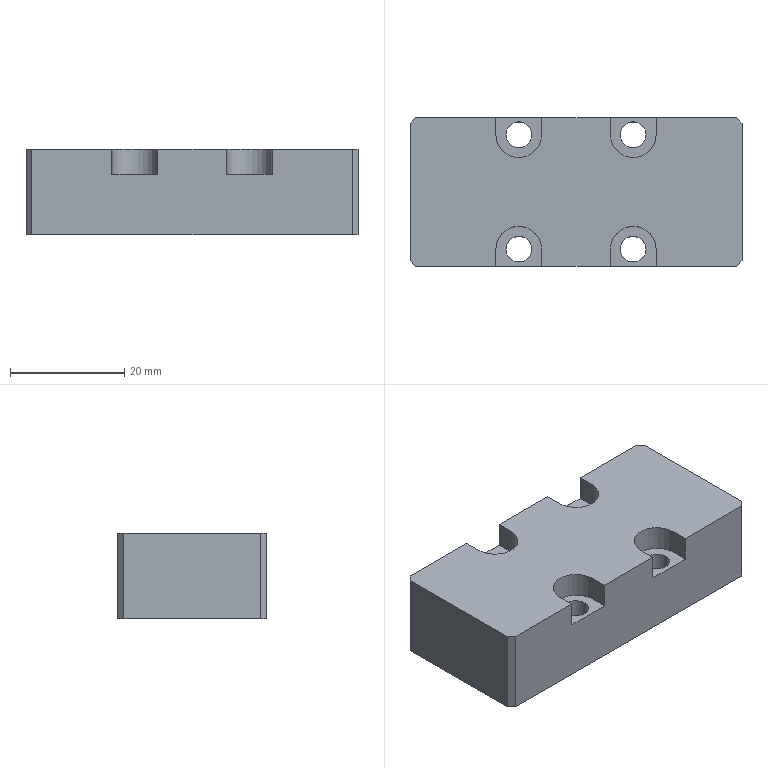Part | SolidWorks | features HoleWzd 2, Chamfer 1, Extrusion 1, ICE 1, MirrorPattern 1 | 1 solid | 42 faces | box 58 x 26 x 15 mm | volume 20953 mm3 | plane 22 | cylinder 16 | cone 4 | commonest cylinder face diameters 4.5 x8 5 x4 8 x4
STEP:
#1=CARTESIAN_POINT('',(15.,0.,-5.5));
#2=VERTEX_POINT('',#1);
#3=CARTESIAN_POINT('',(10.,0.,-5.5));
#4=VERTEX_POINT('',#3);
#5=CARTESIAN_POINT('',(12.5,0.,-5.5));
#6=DIRECTION('',(0.,0.,-1.));
#7=DIRECTION('',(-1.,0.,0.));
#8=AXIS2_PLACEMENT_3D('',#5,#6,#7);
#9=CIRCLE('',#8,2.5);
#10=EDGE_CURVE('',#2,#4,#9,.T.);
#11=ORIENTED_EDGE('',*,*,#10,.F.);
#12=CARTESIAN_POINT('',(15.,0.,-7.5));
#13=VERTEX_POINT('',#12);
#14=CARTESIAN_POINT('',(15.,0.,-7.5));
#15=DIRECTION('',(0.,0.,-1.));
#16=VECTOR('',#15,1000.);
#17=LINE('',#14,#16);
#18=EDGE_CURVE('',#2,#13,#17,.T.);
#19=ORIENTED_EDGE('',*,*,#18,.T.);
#20=CARTESIAN_POINT('',(10.,0.,-7.5));
#21=VERTEX_POINT('',#20);
#22=CARTESIAN_POINT('',(12.5,0.,-7.5));
#23=DIRECTION('',(0.,0.,-1.));
#24=DIRECTION('',(-1.,0.,0.));
#25=AXIS2_PLACEMENT_3D('',#22,#23,#24);
#26=CIRCLE('',#25,2.5);
#27=EDGE_CURVE('',#13,#21,#26,.T.);
#28=ORIENTED_EDGE('',*,*,#27,.T.);
#29=CARTESIAN_POINT('',(10.,0.,-7.5));
#30=DIRECTION('',(0.,0.,-1.));
#31=VECTOR('',#30,1000.);
#32=LINE('',#29,#31);
#33=EDGE_CURVE('',#4,#21,#32,.T.);
#34=ORIENTED_EDGE('',*,*,#33,.F.);
#35=EDGE_LOOP('',(#11,#19,#28,#34));
#36=FACE_OUTER_BOUND('',#35,.T.);
#37=CARTESIAN_POINT('',(12.5,0.,-7.5));
#38=DIRECTION('',(0.,0.,-1.));
#39=DIRECTION('',(-1.,0.,0.));
#40=AXIS2_PLACEMENT_3D('',#37,#38,#39);
#41=CYLINDRICAL_SURFACE('',#40,2.5);
#42=ADVANCED_FACE('',(#36),#41,.F.);
#43=CARTESIAN_POINT('',(12.5,0.,-3.998));
#44=VERTEX_POINT('',#43);
#45=CARTESIAN_POINT('',(10.,0.,-5.5));
#46=DIRECTION('',(-0.8572,0.,-0.515));
#47=VECTOR('',#46,1000.);
#48=LINE('',#45,#47);
#49=EDGE_CURVE('',#44,#4,#48,.T.);
#50=ORIENTED_EDGE('',*,*,#49,.F.);
#51=CARTESIAN_POINT('',(15.,0.,-5.5));
#52=DIRECTION('',(0.8572,0.,-0.515));
#53=VECTOR('',#52,1000.);
#54=LINE('',#51,#53);
#55=EDGE_CURVE('',#44,#2,#54,.T.);
#56=ORIENTED_EDGE('',*,*,#55,.T.);
#57=ORIENTED_EDGE('',*,*,#10,.T.);
#58=EDGE_LOOP('',(#50,#56,#57));
#59=FACE_OUTER_BOUND('',#58,.T.);
#60=CARTESIAN_POINT('',(12.5,0.,-5.5));
#61=DIRECTION('',(0.,0.,-1.));
#62=DIRECTION('',(-1.,0.,0.));
#63=AXIS2_PLACEMENT_3D('',#60,#61,#62);
#64=CONICAL_SURFACE('',#63,2.5,1.03);
#65=ADVANCED_FACE('',(#59),#64,.F.);
#66=CARTESIAN_POINT('',(-10.,0.,-5.5));
#67=VERTEX_POINT('',#66);
#68=CARTESIAN_POINT('',(-15.,0.,-5.5));
#69=VERTEX_POINT('',#68);
#70=CARTESIAN_POINT('',(-12.5,0.,-5.5));
#71=DIRECTION('',(0.,0.,-1.));
#72=DIRECTION('',(-1.,0.,0.));
#73=AXIS2_PLACEMENT_3D('',#70,#71,#72);
#74=CIRCLE('',#73,2.5);
#75=EDGE_CURVE('',#67,#69,#74,.T.);
#76=ORIENTED_EDGE('',*,*,#75,.F.);
#77=CARTESIAN_POINT('',(-10.,0.,-7.5));
#78=VERTEX_POINT('',#77);
#79=CARTESIAN_POINT('',(-10.,0.,-7.5));
#80=DIRECTION('',(0.,0.,-1.));
#81=VECTOR('',#80,1000.);
#82=LINE('',#79,#81);
#83=EDGE_CURVE('',#67,#78,#82,.T.);
#84=ORIENTED_EDGE('',*,*,#83,.T.);
#85=CARTESIAN_POINT('',(-15.,0.,-7.5));
#86=VERTEX_POINT('',#85);
#87=CARTESIAN_POINT('',(-12.5,0.,-7.5));
#88=DIRECTION('',(0.,0.,-1.));
#89=DIRECTION('',(-1.,0.,0.));
#90=AXIS2_PLACEMENT_3D('',#87,#88,#89);
#91=CIRCLE('',#90,2.5);
#92=EDGE_CURVE('',#78,#86,#91,.T.);
#93=ORIENTED_EDGE('',*,*,#92,.T.);
#94=CARTESIAN_POINT('',(-15.,0.,-7.5));
#95=DIRECTION('',(0.,0.,-1.));
#96=VECTOR('',#95,1000.);
#97=LINE('',#94,#96);
#98=EDGE_CURVE('',#69,#86,#97,.T.);
#99=ORIENTED_EDGE('',*,*,#98,.F.);
#100=EDGE_LOOP('',(#76,#84,#93,#99));
#101=FACE_OUTER_BOUND('',#100,.T.);
#102=CARTESIAN_POINT('',(-12.5,0.,-7.5));
#103=DIRECTION('',(0.,0.,-1.));
#104=DIRECTION('',(-1.,0.,0.));
#105=AXIS2_PLACEMENT_3D('',#102,#103,#104);
#106=CYLINDRICAL_SURFACE('',#105,2.5);
#107=ADVANCED_FACE('',(#101),#106,.F.);
#108=CARTESIAN_POINT('',(-12.5,0.,-3.998));
#109=VERTEX_POINT('',#108);
#110=CARTESIAN_POINT('',(-15.,0.,-5.5));
#111=DIRECTION('',(-0.8572,0.,-0.515));
#112=VECTOR('',#111,1000.);
#113=LINE('',#110,#112);
#114=EDGE_CURVE('',#109,#69,#113,.T.);
#115=ORIENTED_EDGE('',*,*,#114,.F.);
#116=CARTESIAN_POINT('',(-10.,0.,-5.5));
#117=DIRECTION('',(0.8572,0.,-0.515));
#118=VECTOR('',#117,1000.);
#119=LINE('',#116,#118);
#120=EDGE_CURVE('',#109,#67,#119,.T.);
#121=ORIENTED_EDGE('',*,*,#120,.T.);
#122=ORIENTED_EDGE('',*,*,#75,.T.);
#123=EDGE_LOOP('',(#115,#121,#122));
#124=FACE_OUTER_BOUND('',#123,.T.);
#125=CARTESIAN_POINT('',(-12.5,0.,-5.5));
#126=DIRECTION('',(0.,0.,-1.));
#127=DIRECTION('',(-1.,0.,0.));
#128=AXIS2_PLACEMENT_3D('',#125,#126,#127);
#129=CONICAL_SURFACE('',#128,2.5,1.03);
#130=ADVANCED_FACE('',(#124),#129,.F.);
#131=CARTESIAN_POINT('',(-12.25,10.,-7.5));
#132=VERTEX_POINT('',#131);
#133=CARTESIAN_POINT('',(-7.75,10.,-7.5));
#134=VERTEX_POINT('',#133);
#135=CARTESIAN_POINT('',(-10.,10.,-7.5));
#136=DIRECTION('',(0.,0.,1.));
#137=DIRECTION('',(1.,0.,0.));
#138=AXIS2_PLACEMENT_3D('',#135,#136,#137);
#139=CIRCLE('',#138,2.25);
#140=EDGE_CURVE('',#132,#134,#139,.T.);
#141=ORIENTED_EDGE('',*,*,#140,.F.);
#142=CARTESIAN_POINT('',(-12.25,10.,3.1));
#143=VERTEX_POINT('',#142);
#144=CARTESIAN_POINT('',(-12.25,10.,7.5));
#145=DIRECTION('',(0.,0.,1.));
#146=VECTOR('',#145,1000.);
#147=LINE('',#144,#146);
#148=EDGE_CURVE('',#132,#143,#147,.T.);
#149=ORIENTED_EDGE('',*,*,#148,.T.);
#150=CARTESIAN_POINT('',(-7.75,10.,3.1));
#151=VERTEX_POINT('',#150);
#152=CARTESIAN_POINT('',(-10.,10.,3.1));
#153=DIRECTION('',(0.,0.,1.));
#154=DIRECTION('',(1.,0.,0.));
#155=AXIS2_PLACEMENT_3D('',#152,#153,#154);
#156=CIRCLE('',#155,2.25);
#157=EDGE_CURVE('',#143,#151,#156,.T.);
#158=ORIENTED_EDGE('',*,*,#157,.T.);
#159=CARTESIAN_POINT('',(-7.75,10.,7.5));
#160=DIRECTION('',(0.,0.,1.));
#161=VECTOR('',#160,1000.);
#162=LINE('',#159,#161);
#163=EDGE_CURVE('',#134,#151,#162,.T.);
#164=ORIENTED_EDGE('',*,*,#163,.F.);
#165=EDGE_LOOP('',(#141,#149,#158,#164));
#166=FACE_OUTER_BOUND('',#165,.T.);
#167=CARTESIAN_POINT('',(-10.,10.,7.5));
#168=DIRECTION('',(0.,0.,1.));
#169=DIRECTION('',(1.,0.,0.));
#170=AXIS2_PLACEMENT_3D('',#167,#168,#169);
#171=CYLINDRICAL_SURFACE('',#170,2.25);
#172=ADVANCED_FACE('',(#166),#171,.F.);
#173=CARTESIAN_POINT('',(-12.25,-10.,-7.5));
#174=VERTEX_POINT('',#173);
#175=CARTESIAN_POINT('',(-7.75,-10.,-7.5));
#176=VERTEX_POINT('',#175);
#177=CARTESIAN_POINT('',(-10.,-10.,-7.5));
#178=DIRECTION('',(0.,0.,1.));
#179=DIRECTION('',(1.,0.,0.));
#180=AXIS2_PLACEMENT_3D('',#177,#178,#179);
#181=CIRCLE('',#180,2.25);
#182=EDGE_CURVE('',#174,#176,#181,.T.);
#183=ORIENTED_EDGE('',*,*,#182,.F.);
#184=CARTESIAN_POINT('',(-12.25,-10.,3.1));
#185=VERTEX_POINT('',#184);
#186=CARTESIAN_POINT('',(-12.25,-10.,7.5));
#187=DIRECTION('',(0.,0.,1.));
#188=VECTOR('',#187,1000.);
#189=LINE('',#186,#188);
#190=EDGE_CURVE('',#174,#185,#189,.T.);
#191=ORIENTED_EDGE('',*,*,#190,.T.);
#192=CARTESIAN_POINT('',(-7.75,-10.,3.1));
#193=VERTEX_POINT('',#192);
#194=CARTESIAN_POINT('',(-10.,-10.,3.1));
#195=DIRECTION('',(0.,0.,1.));
#196=DIRECTION('',(1.,0.,0.));
#197=AXIS2_PLACEMENT_3D('',#194,#195,#196);
#198=CIRCLE('',#197,2.25);
#199=EDGE_CURVE('',#185,#193,#198,.T.);
#200=ORIENTED_EDGE('',*,*,#199,.T.);
#201=CARTESIAN_POINT('',(-7.75,-10.,7.5));
#202=DIRECTION('',(0.,0.,1.));
#203=VECTOR('',#202,1000.);
#204=LINE('',#201,#203);
#205=EDGE_CURVE('',#176,#193,#204,.T.);
#206=ORIENTED_EDGE('',*,*,#205,.F.);
#207=EDGE_LOOP('',(#183,#191,#200,#206));
#208=FACE_OUTER_BOUND('',#207,.T.);
#209=CARTESIAN_POINT('',(-10.,-10.,7.5));
#210=DIRECTION('',(0.,0.,1.));
#211=DIRECTION('',(1.,0.,0.));
#212=AXIS2_PLACEMENT_3D('',#209,#210,#211);
#213=CYLINDRICAL_SURFACE('',#212,2.25);
#214=ADVANCED_FACE('',(#208),#213,.F.);
#215=CARTESIAN_POINT('',(7.75,-10.,-7.5));
#216=VERTEX_POINT('',#215);
#217=CARTESIAN_POINT('',(12.25,-10.,-7.5));
#218=VERTEX_POINT('',#217);
#219=CARTESIAN_POINT('',(10.,-10.,-7.5));
#220=DIRECTION('',(0.,0.,1.));
#221=DIRECTION('',(1.,0.,0.));
#222=AXIS2_PLACEMENT_3D('',#219,#220,#221);
#223=CIRCLE('',#222,2.25);
#224=EDGE_CURVE('',#216,#218,#223,.T.);
#225=ORIENTED_EDGE('',*,*,#224,.F.);
#226=CARTESIAN_POINT('',(7.75,-10.,3.1));
#227=VERTEX_POINT('',#226);
#228=CARTESIAN_POINT('',(7.75,-10.,7.5));
#229=DIRECTION('',(0.,0.,1.));
#230=VECTOR('',#229,1000.);
#231=LINE('',#228,#230);
#232=EDGE_CURVE('',#216,#227,#231,.T.);
#233=ORIENTED_EDGE('',*,*,#232,.T.);
#234=CARTESIAN_POINT('',(12.25,-10.,3.1));
#235=VERTEX_POINT('',#234);
#236=CARTESIAN_POINT('',(10.,-10.,3.1));
#237=DIRECTION('',(0.,0.,1.));
#238=DIRECTION('',(1.,0.,0.));
#239=AXIS2_PLACEMENT_3D('',#236,#237,#238);
#240=CIRCLE('',#239,2.25);
#241=EDGE_CURVE('',#227,#235,#240,.T.);
#242=ORIENTED_EDGE('',*,*,#241,.T.);
#243=CARTESIAN_POINT('',(12.25,-10.,7.5));
#244=DIRECTION('',(0.,0.,1.));
#245=VECTOR('',#244,1000.);
#246=LINE('',#243,#245);
#247=EDGE_CURVE('',#218,#235,#246,.T.);
#248=ORIENTED_EDGE('',*,*,#247,.F.);
#249=EDGE_LOOP('',(#225,#233,#242,#248));
#250=FACE_OUTER_BOUND('',#249,.T.);
#251=CARTESIAN_POINT('',(10.,-10.,7.5));
#252=DIRECTION('',(0.,0.,1.));
#253=DIRECTION('',(1.,0.,0.));
#254=AXIS2_PLACEMENT_3D('',#251,#252,#253);
#255=CYLINDRICAL_SURFACE('',#254,2.25);
#256=ADVANCED_FACE('',(#250),#255,.F.);
#257=CARTESIAN_POINT('',(7.75,10.,-7.5));
#258=VERTEX_POINT('',#257);
#259=CARTESIAN_POINT('',(12.25,10.,-7.5));
#260=VERTEX_POINT('',#259);
#261=CARTESIAN_POINT('',(10.,10.,-7.5));
#262=DIRECTION('',(0.,0.,1.));
#263=DIRECTION('',(1.,0.,0.));
#264=AXIS2_PLACEMENT_3D('',#261,#262,#263);
#265=CIRCLE('',#264,2.25);
#266=EDGE_CURVE('',#258,#260,#265,.T.);
#267=ORIENTED_EDGE('',*,*,#266,.F.);
#268=CARTESIAN_POINT('',(7.75,10.,3.1));
#269=VERTEX_POINT('',#268);
#270=CARTESIAN_POINT('',(7.75,10.,7.5));
#271=DIRECTION('',(0.,0.,1.));
#272=VECTOR('',#271,1000.);
#273=LINE('',#270,#272);
#274=EDGE_CURVE('',#258,#269,#273,.T.);
#275=ORIENTED_EDGE('',*,*,#274,.T.);
#276=CARTESIAN_POINT('',(12.25,10.,3.1));
#277=VERTEX_POINT('',#276);
#278=CARTESIAN_POINT('',(10.,10.,3.1));
#279=DIRECTION('',(0.,0.,1.));
#280=DIRECTION('',(1.,0.,0.));
#281=AXIS2_PLACEMENT_3D('',#278,#279,#280);
#282=CIRCLE('',#281,2.25);
#283=EDGE_CURVE('',#269,#277,#282,.T.);
#284=ORIENTED_EDGE('',*,*,#283,.T.);
#285=CARTESIAN_POINT('',(12.25,10.,7.5));
#286=DIRECTION('',(0.,0.,1.));
#287=VECTOR('',#286,1000.);
#288=LINE('',#285,#287);
#289=EDGE_CURVE('',#260,#277,#288,.T.);
#290=ORIENTED_EDGE('',*,*,#289,.F.);
#291=EDGE_LOOP('',(#267,#275,#284,#290));
#292=FACE_OUTER_BOUND('',#291,.T.);
#293=CARTESIAN_POINT('',(10.,10.,7.5));
#294=DIRECTION('',(0.,0.,1.));
#295=DIRECTION('',(1.,0.,0.));
#296=AXIS2_PLACEMENT_3D('',#293,#294,#295);
#297=CYLINDRICAL_SURFACE('',#296,2.25);
#298=ADVANCED_FACE('',(#292),#297,.F.);
#299=CARTESIAN_POINT('',(-28.,-13.,-7.5));
#300=VERTEX_POINT('',#299);
#301=CARTESIAN_POINT('',(28.,-13.,-7.5));
#302=VERTEX_POINT('',#301);
#303=CARTESIAN_POINT('',(-29.,-13.,-7.5));
#304=DIRECTION('',(1.,0.,0.));
#305=VECTOR('',#304,1000.);
#306=LINE('',#303,#305);
#307=EDGE_CURVE('',#300,#302,#306,.T.);
#308=ORIENTED_EDGE('',*,*,#307,.T.);
#309=CARTESIAN_POINT('',(28.,-13.,7.5));
#310=VERTEX_POINT('',#309);
#311=CARTESIAN_POINT('',(28.,-13.,7.5));
#312=DIRECTION('',(0.,0.,1.));
#313=VECTOR('',#312,1000.);
#314=LINE('',#311,#313);
#315=EDGE_CURVE('',#302,#310,#314,.T.);
#316=ORIENTED_EDGE('',*,*,#315,.T.);
#317=CARTESIAN_POINT('',(14.,-13.,7.5));
#318=VERTEX_POINT('',#317);
#319=CARTESIAN_POINT('',(-29.,-13.,7.5));
#320=DIRECTION('',(1.,0.,0.));
#321=VECTOR('',#320,1000.);
#322=LINE('',#319,#321);
#323=EDGE_CURVE('',#318,#310,#322,.T.);
#324=ORIENTED_EDGE('',*,*,#323,.F.);
#325=CARTESIAN_POINT('',(14.,-13.,3.1));
#326=VERTEX_POINT('',#325);
#327=CARTESIAN_POINT('',(14.,-13.,-5.444));
#328=DIRECTION('',(0.,0.,1.));
#329=VECTOR('',#328,1000.);
#330=LINE('',#327,#329);
#331=EDGE_CURVE('',#326,#318,#330,.T.);
#332=ORIENTED_EDGE('',*,*,#331,.F.);
#333=CARTESIAN_POINT('',(6.,-13.,3.1));
#334=VERTEX_POINT('',#333);
#335=CARTESIAN_POINT('',(-29.,-13.,3.1));
#336=DIRECTION('',(-1.,0.,0.));
#337=VECTOR('',#336,1000.);
#338=LINE('',#335,#337);
#339=EDGE_CURVE('',#326,#334,#338,.T.);
#340=ORIENTED_EDGE('',*,*,#339,.T.);
#341=CARTESIAN_POINT('',(6.,-13.,7.5));
#342=VERTEX_POINT('',#341);
#343=CARTESIAN_POINT('',(6.,-13.,-5.444));
#344=DIRECTION('',(0.,0.,1.));
#345=VECTOR('',#344,1000.);
#346=LINE('',#343,#345);
#347=EDGE_CURVE('',#334,#342,#346,.T.);
#348=ORIENTED_EDGE('',*,*,#347,.T.);
#349=CARTESIAN_POINT('',(-6.,-13.,7.5));
#350=VERTEX_POINT('',#349);
#351=CARTESIAN_POINT('',(-29.,-13.,7.5));
#352=DIRECTION('',(1.,0.,0.));
#353=VECTOR('',#352,1000.);
#354=LINE('',#351,#353);
#355=EDGE_CURVE('',#350,#342,#354,.T.);
#356=ORIENTED_EDGE('',*,*,#355,.F.);
#357=CARTESIAN_POINT('',(-6.,-13.,3.1));
#358=VERTEX_POINT('',#357);
#359=CARTESIAN_POINT('',(-6.,-13.,-5.444));
#360=DIRECTION('',(0.,0.,1.));
#361=VECTOR('',#360,1000.);
#362=LINE('',#359,#361);
#363=EDGE_CURVE('',#358,#350,#362,.T.);
#364=ORIENTED_EDGE('',*,*,#363,.F.);
#365=CARTESIAN_POINT('',(-14.,-13.,3.1));
#366=VERTEX_POINT('',#365);
#367=CARTESIAN_POINT('',(-29.,-13.,3.1));
#368=DIRECTION('',(-1.,0.,0.));
#369=VECTOR('',#368,1000.);
#370=LINE('',#367,#369);
#371=EDGE_CURVE('',#358,#366,#370,.T.);
#372=ORIENTED_EDGE('',*,*,#371,.T.);
#373=CARTESIAN_POINT('',(-14.,-13.,7.5));
#374=VERTEX_POINT('',#373);
#375=CARTESIAN_POINT('',(-14.,-13.,-5.444));
#376=DIRECTION('',(0.,0.,1.));
#377=VECTOR('',#376,1000.);
#378=LINE('',#375,#377);
#379=EDGE_CURVE('',#366,#374,#378,.T.);
#380=ORIENTED_EDGE('',*,*,#379,.T.);
#381=CARTESIAN_POINT('',(-28.,-13.,7.5));
#382=VERTEX_POINT('',#381);
#383=CARTESIAN_POINT('',(-29.,-13.,7.5));
#384=DIRECTION('',(1.,0.,0.));
#385=VECTOR('',#384,1000.);
#386=LINE('',#383,#385);
#387=EDGE_CURVE('',#382,#374,#386,.T.);
#388=ORIENTED_EDGE('',*,*,#387,.F.);
#389=CARTESIAN_POINT('',(-28.,-13.,7.5));
#390=DIRECTION('',(0.,0.,-1.));
#391=VECTOR('',#390,1000.);
#392=LINE('',#389,#391);
#393=EDGE_CURVE('',#382,#300,#392,.T.);
#394=ORIENTED_EDGE('',*,*,#393,.T.);
#395=EDGE_LOOP('',(#308,#316,#324,#332,#340,#348,#356,#364,#372,#380,#388,#394));
#396=FACE_OUTER_BOUND('',#395,.T.);
#397=CARTESIAN_POINT('',(-29.,-13.,7.5));
#398=DIRECTION('',(0.,1.,0.));
#399=DIRECTION('',(0.,0.,1.));
#400=AXIS2_PLACEMENT_3D('',#397,#398,#399);
#401=PLANE('',#400);
#402=ADVANCED_FACE('',(#396),#401,.F.);
#403=ORIENTED_EDGE('',*,*,#323,.T.);
#404=CARTESIAN_POINT('',(29.,-12.,7.5));
#405=VERTEX_POINT('',#404);
#406=CARTESIAN_POINT('',(20.5,-20.5,7.5));
#407=DIRECTION('',(0.7071,0.7071,0.));
#408=VECTOR('',#407,1000.);
#409=LINE('',#406,#408);
#410=EDGE_CURVE('',#310,#405,#409,.T.);
#411=ORIENTED_EDGE('',*,*,#410,.T.);
#412=CARTESIAN_POINT('',(29.,12.,7.5));
#413=VERTEX_POINT('',#412);
#414=CARTESIAN_POINT('',(29.,13.,7.5));
#415=DIRECTION('',(0.,1.,0.));
#416=VECTOR('',#415,1000.);
#417=LINE('',#414,#416);
#418=EDGE_CURVE('',#405,#413,#417,.T.);
#419=ORIENTED_EDGE('',*,*,#418,.T.);
#420=CARTESIAN_POINT('',(28.,13.,7.5));
#421=VERTEX_POINT('',#420);
#422=CARTESIAN_POINT('',(20.5,20.5,7.5));
#423=DIRECTION('',(-0.7071,0.7071,0.));
#424=VECTOR('',#423,1000.);
#425=LINE('',#422,#424);
#426=EDGE_CURVE('',#413,#421,#425,.T.);
#427=ORIENTED_EDGE('',*,*,#426,.T.);
#428=CARTESIAN_POINT('',(14.,13.,7.5));
#429=VERTEX_POINT('',#428);
#430=CARTESIAN_POINT('',(-29.,13.,7.5));
#431=DIRECTION('',(-1.,0.,0.));
#432=VECTOR('',#431,1000.);
#433=LINE('',#430,#432);
#434=EDGE_CURVE('',#421,#429,#433,.T.);
#435=ORIENTED_EDGE('',*,*,#434,.T.);
#436=CARTESIAN_POINT('',(14.,10.,7.5));
#437=VERTEX_POINT('',#436);
#438=CARTESIAN_POINT('',(14.,13.,7.5));
#439=DIRECTION('',(0.,1.,0.));
#440=VECTOR('',#439,1000.);
#441=LINE('',#438,#440);
#442=EDGE_CURVE('',#437,#429,#441,.T.);
#443=ORIENTED_EDGE('',*,*,#442,.F.);
#444=CARTESIAN_POINT('',(6.,10.,7.5));
#445=VERTEX_POINT('',#444);
#446=CARTESIAN_POINT('',(10.,10.,7.5));
#447=DIRECTION('',(0.,0.,1.));
#448=DIRECTION('',(1.,0.,0.));
#449=AXIS2_PLACEMENT_3D('',#446,#447,#448);
#450=CIRCLE('',#449,4.);
#451=EDGE_CURVE('',#445,#437,#450,.T.);
#452=ORIENTED_EDGE('',*,*,#451,.F.);
#453=CARTESIAN_POINT('',(6.,13.,7.5));
#454=VERTEX_POINT('',#453);
#455=CARTESIAN_POINT('',(6.,13.,7.5));
#456=DIRECTION('',(0.,-1.,0.));
#457=VECTOR('',#456,1000.);
#458=LINE('',#455,#457);
#459=EDGE_CURVE('',#454,#445,#458,.T.);
#460=ORIENTED_EDGE('',*,*,#459,.F.);
#461=CARTESIAN_POINT('',(-6.,13.,7.5));
#462=VERTEX_POINT('',#461);
#463=CARTESIAN_POINT('',(-29.,13.,7.5));
#464=DIRECTION('',(-1.,0.,0.));
#465=VECTOR('',#464,1000.);
#466=LINE('',#463,#465);
#467=EDGE_CURVE('',#454,#462,#466,.T.);
#468=ORIENTED_EDGE('',*,*,#467,.T.);
#469=CARTESIAN_POINT('',(-6.,10.,7.5));
#470=VERTEX_POINT('',#469);
#471=CARTESIAN_POINT('',(-6.,13.,7.5));
#472=DIRECTION('',(0.,1.,0.));
#473=VECTOR('',#472,1000.);
#474=LINE('',#471,#473);
#475=EDGE_CURVE('',#470,#462,#474,.T.);
#476=ORIENTED_EDGE('',*,*,#475,.F.);
#477=CARTESIAN_POINT('',(-14.,10.,7.5));
#478=VERTEX_POINT('',#477);
#479=CARTESIAN_POINT('',(-10.,10.,7.5));
#480=DIRECTION('',(0.,0.,1.));
#481=DIRECTION('',(1.,0.,0.));
#482=AXIS2_PLACEMENT_3D('',#479,#480,#481);
#483=CIRCLE('',#482,4.);
#484=EDGE_CURVE('',#478,#470,#483,.T.);
#485=ORIENTED_EDGE('',*,*,#484,.F.);
#486=CARTESIAN_POINT('',(-14.,13.,7.5));
#487=VERTEX_POINT('',#486);
#488=CARTESIAN_POINT('',(-14.,13.,7.5));
#489=DIRECTION('',(0.,-1.,0.));
#490=VECTOR('',#489,1000.);
#491=LINE('',#488,#490);
#492=EDGE_CURVE('',#487,#478,#491,.T.);
#493=ORIENTED_EDGE('',*,*,#492,.F.);
#494=CARTESIAN_POINT('',(-28.,13.,7.5));
#495=VERTEX_POINT('',#494);
#496=CARTESIAN_POINT('',(-29.,13.,7.5));
#497=DIRECTION('',(-1.,0.,0.));
#498=VECTOR('',#497,1000.);
#499=LINE('',#496,#498);
#500=EDGE_CURVE('',#487,#495,#499,.T.);
#501=ORIENTED_EDGE('',*,*,#500,.T.);
#502=CARTESIAN_POINT('',(-29.,12.,7.5));
#503=VERTEX_POINT('',#502);
#504=CARTESIAN_POINT('',(-20.5,20.5,7.5));
#505=DIRECTION('',(-0.7071,-0.7071,0.));
#506=VECTOR('',#505,1000.);
#507=LINE('',#504,#506);
#508=EDGE_CURVE('',#495,#503,#507,.T.);
#509=ORIENTED_EDGE('',*,*,#508,.T.);
#510=CARTESIAN_POINT('',(-29.,-12.,7.5));
#511=VERTEX_POINT('',#510);
#512=CARTESIAN_POINT('',(-29.,13.,7.5));
#513=DIRECTION('',(0.,-1.,0.));
#514=VECTOR('',#513,1000.);
#515=LINE('',#512,#514);
#516=EDGE_CURVE('',#503,#511,#515,.T.);
#517=ORIENTED_EDGE('',*,*,#516,.T.);
#518=CARTESIAN_POINT('',(-20.5,-20.5,7.5));
#519=DIRECTION('',(0.7071,-0.7071,0.));
#520=VECTOR('',#519,1000.);
#521=LINE('',#518,#520);
#522=EDGE_CURVE('',#511,#382,#521,.T.);
#523=ORIENTED_EDGE('',*,*,#522,.T.);
#524=ORIENTED_EDGE('',*,*,#387,.T.);
#525=CARTESIAN_POINT('',(-14.,-10.,7.5));
#526=VERTEX_POINT('',#525);
#527=CARTESIAN_POINT('',(-14.,-13.,7.5));
#528=DIRECTION('',(0.,1.,0.));
#529=VECTOR('',#528,1000.);
#530=LINE('',#527,#529);
#531=EDGE_CURVE('',#374,#526,#530,.T.);
#532=ORIENTED_EDGE('',*,*,#531,.T.);
#533=CARTESIAN_POINT('',(-6.,-10.,7.5));
#534=VERTEX_POINT('',#533);
#535=CARTESIAN_POINT('',(-10.,-10.,7.5));
#536=DIRECTION('',(0.,0.,1.));
#537=DIRECTION('',(1.,0.,0.));
#538=AXIS2_PLACEMENT_3D('',#535,#536,#537);
#539=CIRCLE('',#538,4.);
#540=EDGE_CURVE('',#534,#526,#539,.T.);
#541=ORIENTED_EDGE('',*,*,#540,.F.);
#542=CARTESIAN_POINT('',(-6.,-13.,7.5));
#543=DIRECTION('',(0.,-1.,0.));
#544=VECTOR('',#543,1000.);
#545=LINE('',#542,#544);
#546=EDGE_CURVE('',#534,#350,#545,.T.);
#547=ORIENTED_EDGE('',*,*,#546,.T.);
#548=ORIENTED_EDGE('',*,*,#355,.T.);
#549=CARTESIAN_POINT('',(6.,-10.,7.5));
#550=VERTEX_POINT('',#549);
#551=CARTESIAN_POINT('',(6.,-13.,7.5));
#552=DIRECTION('',(0.,1.,0.));
#553=VECTOR('',#552,1000.);
#554=LINE('',#551,#553);
#555=EDGE_CURVE('',#342,#550,#554,.T.);
#556=ORIENTED_EDGE('',*,*,#555,.T.);
#557=CARTESIAN_POINT('',(14.,-10.,7.5));
#558=VERTEX_POINT('',#557);
#559=CARTESIAN_POINT('',(10.,-10.,7.5));
#560=DIRECTION('',(0.,0.,1.));
#561=DIRECTION('',(1.,0.,0.));
#562=AXIS2_PLACEMENT_3D('',#559,#560,#561);
#563=CIRCLE('',#562,4.);
#564=EDGE_CURVE('',#558,#550,#563,.T.);
#565=ORIENTED_EDGE('',*,*,#564,.F.);
#566=CARTESIAN_POINT('',(14.,-13.,7.5));
#567=DIRECTION('',(0.,-1.,0.));
#568=VECTOR('',#567,1000.);
#569=LINE('',#566,#568);
#570=EDGE_CURVE('',#558,#318,#569,.T.);
#571=ORIENTED_EDGE('',*,*,#570,.T.);
#572=EDGE_LOOP('',(#403,#411,#419,#427,#435,#443,#452,#460,#468,#476,#485,#493,#501,#509,#517,#523,#524,#532,#541,#547,#548,#556,#565,#571));
#573=FACE_OUTER_BOUND('',#572,.T.);
#574=CARTESIAN_POINT('',(0.,0.,7.5));
#575=DIRECTION('',(0.,0.,1.));
#576=DIRECTION('',(1.,0.,0.));
#577=AXIS2_PLACEMENT_3D('',#574,#575,#576);
#578=PLANE('',#577);
#579=ADVANCED_FACE('',(#573),#578,.T.);
#580=CARTESIAN_POINT('',(14.,-10.,3.1));
#581=VERTEX_POINT('',#580);
#582=CARTESIAN_POINT('',(14.,-10.,-5.444));
#583=DIRECTION('',(0.,0.,1.));
#584=VECTOR('',#583,1000.);
#585=LINE('',#582,#584);
#586=EDGE_CURVE('',#581,#558,#585,.T.);
#587=ORIENTED_EDGE('',*,*,#586,.T.);
#588=ORIENTED_EDGE('',*,*,#564,.T.);
#589=CARTESIAN_POINT('',(6.,-10.,3.1));
#590=VERTEX_POINT('',#589);
#591=CARTESIAN_POINT('',(6.,-10.,-5.444));
#592=DIRECTION('',(0.,0.,1.));
#593=VECTOR('',#592,1000.);
#594=LINE('',#591,#593);
#595=EDGE_CURVE('',#590,#550,#594,.T.);
#596=ORIENTED_EDGE('',*,*,#595,.F.);
#597=CARTESIAN_POINT('',(10.,-10.,3.1));
#598=DIRECTION('',(0.,0.,1.));
#599=DIRECTION('',(1.,0.,0.));
#600=AXIS2_PLACEMENT_3D('',#597,#598,#599);
#601=CIRCLE('',#600,4.);
#602=EDGE_CURVE('',#581,#590,#601,.T.);
#603=ORIENTED_EDGE('',*,*,#602,.F.);
#604=EDGE_LOOP('',(#587,#588,#596,#603));
#605=FACE_OUTER_BOUND('',#604,.T.);
#606=CARTESIAN_POINT('',(10.,-10.,7.5));
#607=DIRECTION('',(0.,0.,1.));
#608=DIRECTION('',(1.,0.,0.));
#609=AXIS2_PLACEMENT_3D('',#606,#607,#608);
#610=CYLINDRICAL_SURFACE('',#609,4.);
#611=ADVANCED_FACE('',(#605),#610,.F.);
#612=CARTESIAN_POINT('',(-6.,-10.,3.1));
#613=VERTEX_POINT('',#612);
#614=CARTESIAN_POINT('',(-6.,-10.,-5.444));
#615=DIRECTION('',(0.,0.,1.));
#616=VECTOR('',#615,1000.);
#617=LINE('',#614,#616);
#618=EDGE_CURVE('',#613,#534,#617,.T.);
#619=ORIENTED_EDGE('',*,*,#618,.T.);
#620=ORIENTED_EDGE('',*,*,#540,.T.);
#621=CARTESIAN_POINT('',(-14.,-10.,3.1));
#622=VERTEX_POINT('',#621);
#623=CARTESIAN_POINT('',(-14.,-10.,-5.444));
#624=DIRECTION('',(0.,0.,1.));
#625=VECTOR('',#624,1000.);
#626=LINE('',#623,#625);
#627=EDGE_CURVE('',#622,#526,#626,.T.);
#628=ORIENTED_EDGE('',*,*,#627,.F.);
#629=CARTESIAN_POINT('',(-10.,-10.,3.1));
#630=DIRECTION('',(0.,0.,1.));
#631=DIRECTION('',(1.,0.,0.));
#632=AXIS2_PLACEMENT_3D('',#629,#630,#631);
#633=CIRCLE('',#632,4.);
#634=EDGE_CURVE('',#613,#622,#633,.T.);
#635=ORIENTED_EDGE('',*,*,#634,.F.);
#636=EDGE_LOOP('',(#619,#620,#628,#635));
#637=FACE_OUTER_BOUND('',#636,.T.);
#638=CARTESIAN_POINT('',(-10.,-10.,7.5));
#639=DIRECTION('',(0.,0.,1.));
#640=DIRECTION('',(1.,0.,0.));
#641=AXIS2_PLACEMENT_3D('',#638,#639,#640);
#642=CYLINDRICAL_SURFACE('',#641,4.);
#643=ADVANCED_FACE('',(#637),#642,.F.);
#644=ORIENTED_EDGE('',*,*,#418,.F.);
#645=CARTESIAN_POINT('',(29.,-12.,-7.5));
#646=VERTEX_POINT('',#645);
#647=CARTESIAN_POINT('',(29.,-12.,7.5));
#648=DIRECTION('',(0.,0.,-1.));
#649=VECTOR('',#648,1000.);
#650=LINE('',#647,#649);
#651=EDGE_CURVE('',#405,#646,#650,.T.);
#652=ORIENTED_EDGE('',*,*,#651,.T.);
#653=CARTESIAN_POINT('',(29.,12.,-7.5));
#654=VERTEX_POINT('',#653);
#655=CARTESIAN_POINT('',(29.,13.,-7.5));
#656=DIRECTION('',(0.,1.,0.));
#657=VECTOR('',#656,1000.);
#658=LINE('',#655,#657);
#659=EDGE_CURVE('',#646,#654,#658,.T.);
#660=ORIENTED_EDGE('',*,*,#659,.T.);
#661=CARTESIAN_POINT('',(29.,12.,7.5));
#662=DIRECTION('',(0.,0.,1.));
#663=VECTOR('',#662,1000.);
#664=LINE('',#661,#663);
#665=EDGE_CURVE('',#654,#413,#664,.T.);
#666=ORIENTED_EDGE('',*,*,#665,.T.);
#667=EDGE_LOOP('',(#644,#652,#660,#666));
#668=FACE_OUTER_BOUND('',#667,.T.);
#669=CARTESIAN_POINT('',(29.,13.,7.5));
#670=DIRECTION('',(-1.,0.,0.));
#671=DIRECTION('',(0.,-1.,0.));
#672=AXIS2_PLACEMENT_3D('',#669,#670,#671);
#673=PLANE('',#672);
#674=ADVANCED_FACE('',(#668),#673,.F.);
#675=ORIENTED_EDGE('',*,*,#434,.F.);
#676=CARTESIAN_POINT('',(28.,13.,-7.5));
#677=VERTEX_POINT('',#676);
#678=CARTESIAN_POINT('',(28.,13.,7.5));
#679=DIRECTION('',(0.,0.,-1.));
#680=VECTOR('',#679,1000.);
#681=LINE('',#678,#680);
#682=EDGE_CURVE('',#421,#677,#681,.T.);
#683=ORIENTED_EDGE('',*,*,#682,.T.);
#684=CARTESIAN_POINT('',(-28.,13.,-7.5));
#685=VERTEX_POINT('',#684);
#686=CARTESIAN_POINT('',(-29.,13.,-7.5));
#687=DIRECTION('',(-1.,0.,0.));
#688=VECTOR('',#687,1000.);
#689=LINE('',#686,#688);
#690=EDGE_CURVE('',#677,#685,#689,.T.);
#691=ORIENTED_EDGE('',*,*,#690,.T.);
#692=CARTESIAN_POINT('',(-28.,13.,7.5));
#693=DIRECTION('',(0.,0.,1.));
#694=VECTOR('',#693,1000.);
#695=LINE('',#692,#694);
#696=EDGE_CURVE('',#685,#495,#695,.T.);
#697=ORIENTED_EDGE('',*,*,#696,.T.);
#698=ORIENTED_EDGE('',*,*,#500,.F.);
#699=CARTESIAN_POINT('',(-14.,13.,3.1));
#700=VERTEX_POINT('',#699);
#701=CARTESIAN_POINT('',(-14.,13.,-5.444));
#702=DIRECTION('',(0.,0.,1.));
#703=VECTOR('',#702,1000.);
#704=LINE('',#701,#703);
#705=EDGE_CURVE('',#700,#487,#704,.T.);
#706=ORIENTED_EDGE('',*,*,#705,.F.);
#707=CARTESIAN_POINT('',(-6.,13.,3.1));
#708=VERTEX_POINT('',#707);
#709=CARTESIAN_POINT('',(-29.,13.,3.1));
#710=DIRECTION('',(1.,0.,0.));
#711=VECTOR('',#710,1000.);
#712=LINE('',#709,#711);
#713=EDGE_CURVE('',#700,#708,#712,.T.);
#714=ORIENTED_EDGE('',*,*,#713,.T.);
#715=CARTESIAN_POINT('',(-6.,13.,-5.444));
#716=DIRECTION('',(0.,0.,1.));
#717=VECTOR('',#716,1000.);
#718=LINE('',#715,#717);
#719=EDGE_CURVE('',#708,#462,#718,.T.);
#720=ORIENTED_EDGE('',*,*,#719,.T.);
#721=ORIENTED_EDGE('',*,*,#467,.F.);
#722=CARTESIAN_POINT('',(6.,13.,3.1));
#723=VERTEX_POINT('',#722);
#724=CARTESIAN_POINT('',(6.,13.,-5.444));
#725=DIRECTION('',(0.,0.,1.));
#726=VECTOR('',#725,1000.);
#727=LINE('',#724,#726);
#728=EDGE_CURVE('',#723,#454,#727,.T.);
#729=ORIENTED_EDGE('',*,*,#728,.F.);
#730=CARTESIAN_POINT('',(14.,13.,3.1));
#731=VERTEX_POINT('',#730);
#732=CARTESIAN_POINT('',(-29.,13.,3.1));
#733=DIRECTION('',(1.,0.,0.));
#734=VECTOR('',#733,1000.);
#735=LINE('',#732,#734);
#736=EDGE_CURVE('',#723,#731,#735,.T.);
#737=ORIENTED_EDGE('',*,*,#736,.T.);
#738=CARTESIAN_POINT('',(14.,13.,-5.444));
#739=DIRECTION('',(0.,0.,1.));
#740=VECTOR('',#739,1000.);
#741=LINE('',#738,#740);
#742=EDGE_CURVE('',#731,#429,#741,.T.);
#743=ORIENTED_EDGE('',*,*,#742,.T.);
#744=EDGE_LOOP('',(#675,#683,#691,#697,#698,#706,#714,#720,#721,#729,#737,#743));
#745=FACE_OUTER_BOUND('',#744,.T.);
#746=CARTESIAN_POINT('',(-29.,13.,7.5));
#747=DIRECTION('',(0.,-1.,0.));
#748=DIRECTION('',(0.,0.,-1.));
#749=AXIS2_PLACEMENT_3D('',#746,#747,#748);
#750=PLANE('',#749);
#751=ADVANCED_FACE('',(#745),#750,.F.);
#752=ORIENTED_EDGE('',*,*,#516,.F.);
#753=CARTESIAN_POINT('',(-29.,12.,-7.5));
#754=VERTEX_POINT('',#753);
#755=CARTESIAN_POINT('',(-29.,12.,7.5));
#756=DIRECTION('',(0.,0.,-1.));
#757=VECTOR('',#756,1000.);
#758=LINE('',#755,#757);
#759=EDGE_CURVE('',#503,#754,#758,.T.);
#760=ORIENTED_EDGE('',*,*,#759,.T.);
#761=CARTESIAN_POINT('',(-29.,-12.,-7.5));
#762=VERTEX_POINT('',#761);
#763=CARTESIAN_POINT('',(-29.,13.,-7.5));
#764=DIRECTION('',(0.,-1.,0.));
#765=VECTOR('',#764,1000.);
#766=LINE('',#763,#765);
#767=EDGE_CURVE('',#754,#762,#766,.T.);
#768=ORIENTED_EDGE('',*,*,#767,.T.);
#769=CARTESIAN_POINT('',(-29.,-12.,7.5));
#770=DIRECTION('',(0.,0.,1.));
#771=VECTOR('',#770,1000.);
#772=LINE('',#769,#771);
#773=EDGE_CURVE('',#762,#511,#772,.T.);
#774=ORIENTED_EDGE('',*,*,#773,.T.);
#775=EDGE_LOOP('',(#752,#760,#768,#774));
#776=FACE_OUTER_BOUND('',#775,.T.);
#777=CARTESIAN_POINT('',(-29.,13.,7.5));
#778=DIRECTION('',(1.,0.,0.));
#779=DIRECTION('',(0.,1.,0.));
#780=AXIS2_PLACEMENT_3D('',#777,#778,#779);
#781=PLANE('',#780);
#782=ADVANCED_FACE('',(#776),#781,.F.);
#783=CARTESIAN_POINT('',(12.5,0.,-7.5));
#784=DIRECTION('',(0.,0.,-1.));
#785=DIRECTION('',(-1.,0.,0.));
#786=AXIS2_PLACEMENT_3D('',#783,#784,#785);
#787=CIRCLE('',#786,2.5);
#788=EDGE_CURVE('',#21,#13,#787,.T.);
#789=ORIENTED_EDGE('',*,*,#788,.F.);
#790=ORIENTED_EDGE('',*,*,#27,.F.);
#791=EDGE_LOOP('',(#789,#790));
#792=FACE_BOUND('',#791,.T.);
#793=CARTESIAN_POINT('',(-12.5,0.,-7.5));
#794=DIRECTION('',(0.,0.,-1.));
#795=DIRECTION('',(-1.,0.,0.));
#796=AXIS2_PLACEMENT_3D('',#793,#794,#795);
#797=CIRCLE('',#796,2.5);
#798=EDGE_CURVE('',#86,#78,#797,.T.);
#799=ORIENTED_EDGE('',*,*,#798,.F.);
#800=ORIENTED_EDGE('',*,*,#92,.F.);
#801=EDGE_LOOP('',(#799,#800));
#802=FACE_BOUND('',#801,.T.);
#803=CARTESIAN_POINT('',(-10.,10.,-7.5));
#804=DIRECTION('',(0.,0.,1.));
#805=DIRECTION('',(1.,0.,0.));
#806=AXIS2_PLACEMENT_3D('',#803,#804,#805);
#807=CIRCLE('',#806,2.25);
#808=EDGE_CURVE('',#134,#132,#807,.T.);
#809=ORIENTED_EDGE('',*,*,#808,.T.);
#810=ORIENTED_EDGE('',*,*,#140,.T.);
#811=EDGE_LOOP('',(#809,#810));
#812=FACE_BOUND('',#811,.T.);
#813=CARTESIAN_POINT('',(-10.,-10.,-7.5));
#814=DIRECTION('',(0.,0.,1.));
#815=DIRECTION('',(1.,0.,0.));
#816=AXIS2_PLACEMENT_3D('',#813,#814,#815);
#817=CIRCLE('',#816,2.25);
#818=EDGE_CURVE('',#176,#174,#817,.T.);
#819=ORIENTED_EDGE('',*,*,#818,.T.);
#820=ORIENTED_EDGE('',*,*,#182,.T.);
#821=EDGE_LOOP('',(#819,#820));
#822=FACE_BOUND('',#821,.T.);
#823=CARTESIAN_POINT('',(10.,-10.,-7.5));
#824=DIRECTION('',(0.,0.,1.));
#825=DIRECTION('',(1.,0.,0.));
#826=AXIS2_PLACEMENT_3D('',#823,#824,#825);
#827=CIRCLE('',#826,2.25);
#828=EDGE_CURVE('',#218,#216,#827,.T.);
#829=ORIENTED_EDGE('',*,*,#828,.T.);
#830=ORIENTED_EDGE('',*,*,#224,.T.);
#831=EDGE_LOOP('',(#829,#830));
#832=FACE_BOUND('',#831,.T.);
#833=CARTESIAN_POINT('',(10.,10.,-7.5));
#834=DIRECTION('',(0.,0.,1.));
#835=DIRECTION('',(1.,0.,0.));
#836=AXIS2_PLACEMENT_3D('',#833,#834,#835);
#837=CIRCLE('',#836,2.25);
#838=EDGE_CURVE('',#260,#258,#837,.T.);
#839=ORIENTED_EDGE('',*,*,#838,.T.);
#840=ORIENTED_EDGE('',*,*,#266,.T.);
#841=EDGE_LOOP('',(#839,#840));
#842=FACE_BOUND('',#841,.T.);
#843=ORIENTED_EDGE('',*,*,#659,.F.);
#844=CARTESIAN_POINT('',(29.,-12.,-7.5));
#845=DIRECTION('',(-0.7071,-0.7071,0.));
#846=VECTOR('',#845,1000.);
#847=LINE('',#844,#846);
#848=EDGE_CURVE('',#646,#302,#847,.T.);
#849=ORIENTED_EDGE('',*,*,#848,.T.);
#850=ORIENTED_EDGE('',*,*,#307,.F.);
#851=CARTESIAN_POINT('',(-28.,-13.,-7.5));
#852=DIRECTION('',(-0.7071,0.7071,0.));
#853=VECTOR('',#852,1000.);
#854=LINE('',#851,#853);
#855=EDGE_CURVE('',#300,#762,#854,.T.);
#856=ORIENTED_EDGE('',*,*,#855,.T.);
#857=ORIENTED_EDGE('',*,*,#767,.F.);
#858=CARTESIAN_POINT('',(-29.,12.,-7.5));
#859=DIRECTION('',(0.7071,0.7071,0.));
#860=VECTOR('',#859,1000.);
#861=LINE('',#858,#860);
#862=EDGE_CURVE('',#754,#685,#861,.T.);
#863=ORIENTED_EDGE('',*,*,#862,.T.);
#864=ORIENTED_EDGE('',*,*,#690,.F.);
#865=CARTESIAN_POINT('',(28.,13.,-7.5));
#866=DIRECTION('',(0.7071,-0.7071,0.));
#867=VECTOR('',#866,1000.);
#868=LINE('',#865,#867);
#869=EDGE_CURVE('',#677,#654,#868,.T.);
#870=ORIENTED_EDGE('',*,*,#869,.T.);
#871=EDGE_LOOP('',(#843,#849,#850,#856,#857,#863,#864,#870));
#872=FACE_OUTER_BOUND('',#871,.T.);
#873=CARTESIAN_POINT('',(0.,0.,-7.5));
#874=DIRECTION('',(0.,0.,1.));
#875=DIRECTION('',(1.,0.,0.));
#876=AXIS2_PLACEMENT_3D('',#873,#874,#875);
#877=PLANE('',#876);
#878=ADVANCED_FACE('',(#792,#802,#812,#822,#832,#842,#872),#877,.F.);
#879=CARTESIAN_POINT('',(10.,10.,3.1));
#880=DIRECTION('',(0.,0.,1.));
#881=DIRECTION('',(1.,0.,0.));
#882=AXIS2_PLACEMENT_3D('',#879,#880,#881);
#883=CIRCLE('',#882,2.25);
#884=EDGE_CURVE('',#277,#269,#883,.T.);
#885=ORIENTED_EDGE('',*,*,#884,.F.);
#886=ORIENTED_EDGE('',*,*,#283,.F.);
#887=EDGE_LOOP('',(#885,#886));
#888=FACE_BOUND('',#887,.T.);
#889=CARTESIAN_POINT('',(6.,10.,3.1));
#890=VERTEX_POINT('',#889);
#891=CARTESIAN_POINT('',(14.,10.,3.1));
#892=VERTEX_POINT('',#891);
#893=CARTESIAN_POINT('',(10.,10.,3.1));
#894=DIRECTION('',(0.,0.,1.));
#895=DIRECTION('',(1.,0.,0.));
#896=AXIS2_PLACEMENT_3D('',#893,#894,#895);
#897=CIRCLE('',#896,4.);
#898=EDGE_CURVE('',#890,#892,#897,.T.);
#899=ORIENTED_EDGE('',*,*,#898,.T.);
#900=CARTESIAN_POINT('',(14.,13.,3.1));
#901=DIRECTION('',(0.,1.,0.));
#902=VECTOR('',#901,1000.);
#903=LINE('',#900,#902);
#904=EDGE_CURVE('',#892,#731,#903,.T.);
#905=ORIENTED_EDGE('',*,*,#904,.T.);
#906=ORIENTED_EDGE('',*,*,#736,.F.);
#907=CARTESIAN_POINT('',(6.,13.,3.1));
#908=DIRECTION('',(0.,-1.,0.));
#909=VECTOR('',#908,1000.);
#910=LINE('',#907,#909);
#911=EDGE_CURVE('',#723,#890,#910,.T.);
#912=ORIENTED_EDGE('',*,*,#911,.T.);
#913=EDGE_LOOP('',(#899,#905,#906,#912));
#914=FACE_OUTER_BOUND('',#913,.T.);
#915=CARTESIAN_POINT('',(12.25,10.,3.1));
#916=DIRECTION('',(0.,0.,-1.));
#917=DIRECTION('',(-1.,0.,0.));
#918=AXIS2_PLACEMENT_3D('',#915,#916,#917);
#919=PLANE('',#918);
#920=ADVANCED_FACE('',(#888,#914),#919,.F.);
#921=ORIENTED_EDGE('',*,*,#898,.F.);
#922=CARTESIAN_POINT('',(6.,10.,-5.444));
#923=DIRECTION('',(0.,0.,1.));
#924=VECTOR('',#923,1000.);
#925=LINE('',#922,#924);
#926=EDGE_CURVE('',#890,#445,#925,.T.);
#927=ORIENTED_EDGE('',*,*,#926,.T.);
#928=ORIENTED_EDGE('',*,*,#451,.T.);
#929=CARTESIAN_POINT('',(14.,10.,-5.444));
#930=DIRECTION('',(0.,0.,1.));
#931=VECTOR('',#930,1000.);
#932=LINE('',#929,#931);
#933=EDGE_CURVE('',#892,#437,#932,.T.);
#934=ORIENTED_EDGE('',*,*,#933,.F.);
#935=EDGE_LOOP('',(#921,#927,#928,#934));
#936=FACE_OUTER_BOUND('',#935,.T.);
#937=CARTESIAN_POINT('',(10.,10.,7.5));
#938=DIRECTION('',(0.,0.,1.));
#939=DIRECTION('',(1.,0.,0.));
#940=AXIS2_PLACEMENT_3D('',#937,#938,#939);
#941=CYLINDRICAL_SURFACE('',#940,4.);
#942=ADVANCED_FACE('',(#936),#941,.F.);
#943=ORIENTED_EDGE('',*,*,#274,.F.);
#944=ORIENTED_EDGE('',*,*,#838,.F.);
#945=ORIENTED_EDGE('',*,*,#289,.T.);
#946=ORIENTED_EDGE('',*,*,#884,.T.);
#947=EDGE_LOOP('',(#943,#944,#945,#946));
#948=FACE_OUTER_BOUND('',#947,.T.);
#949=CARTESIAN_POINT('',(10.,10.,7.5));
#950=DIRECTION('',(0.,0.,1.));
#951=DIRECTION('',(1.,0.,0.));
#952=AXIS2_PLACEMENT_3D('',#949,#950,#951);
#953=CYLINDRICAL_SURFACE('',#952,2.25);
#954=ADVANCED_FACE('',(#948),#953,.F.);
#955=CARTESIAN_POINT('',(10.,-10.,3.1));
#956=DIRECTION('',(0.,0.,1.));
#957=DIRECTION('',(1.,0.,0.));
#958=AXIS2_PLACEMENT_3D('',#955,#956,#957);
#959=CIRCLE('',#958,2.25);
#960=EDGE_CURVE('',#235,#227,#959,.T.);
#961=ORIENTED_EDGE('',*,*,#960,.F.);
#962=ORIENTED_EDGE('',*,*,#241,.F.);
#963=EDGE_LOOP('',(#961,#962));
#964=FACE_BOUND('',#963,.T.);
#965=ORIENTED_EDGE('',*,*,#339,.F.);
#966=CARTESIAN_POINT('',(14.,-13.,3.1));
#967=DIRECTION('',(0.,-1.,0.));
#968=VECTOR('',#967,1000.);
#969=LINE('',#966,#968);
#970=EDGE_CURVE('',#581,#326,#969,.T.);
#971=ORIENTED_EDGE('',*,*,#970,.F.);
#972=ORIENTED_EDGE('',*,*,#602,.T.);
#973=CARTESIAN_POINT('',(6.,-13.,3.1));
#974=DIRECTION('',(0.,1.,0.));
#975=VECTOR('',#974,1000.);
#976=LINE('',#973,#975);
#977=EDGE_CURVE('',#334,#590,#976,.T.);
#978=ORIENTED_EDGE('',*,*,#977,.F.);
#979=EDGE_LOOP('',(#965,#971,#972,#978));
#980=FACE_OUTER_BOUND('',#979,.T.);
#981=CARTESIAN_POINT('',(12.25,-10.,3.1));
#982=DIRECTION('',(0.,0.,-1.));
#983=DIRECTION('',(-1.,0.,0.));
#984=AXIS2_PLACEMENT_3D('',#981,#982,#983);
#985=PLANE('',#984);
#986=ADVANCED_FACE('',(#964,#980),#985,.F.);
#987=ORIENTED_EDGE('',*,*,#232,.F.);
#988=ORIENTED_EDGE('',*,*,#828,.F.);
#989=ORIENTED_EDGE('',*,*,#247,.T.);
#990=ORIENTED_EDGE('',*,*,#960,.T.);
#991=EDGE_LOOP('',(#987,#988,#989,#990));
#992=FACE_OUTER_BOUND('',#991,.T.);
#993=CARTESIAN_POINT('',(10.,-10.,7.5));
#994=DIRECTION('',(0.,0.,1.));
#995=DIRECTION('',(1.,0.,0.));
#996=AXIS2_PLACEMENT_3D('',#993,#994,#995);
#997=CYLINDRICAL_SURFACE('',#996,2.25);
#998=ADVANCED_FACE('',(#992),#997,.F.);
#999=CARTESIAN_POINT('',(-10.,-10.,3.1));
#1000=DIRECTION('',(0.,0.,1.));
#1001=DIRECTION('',(1.,0.,0.));
#1002=AXIS2_PLACEMENT_3D('',#999,#1000,#1001);
#1003=CIRCLE('',#1002,2.25);
#1004=EDGE_CURVE('',#193,#185,#1003,.T.);
#1005=ORIENTED_EDGE('',*,*,#1004,.F.);
#1006=ORIENTED_EDGE('',*,*,#199,.F.);
#1007=EDGE_LOOP('',(#1005,#1006));
#1008=FACE_BOUND('',#1007,.T.);
#1009=ORIENTED_EDGE('',*,*,#371,.F.);
#1010=CARTESIAN_POINT('',(-6.,-13.,3.1));
#1011=DIRECTION('',(0.,-1.,0.));
#1012=VECTOR('',#1011,1000.);
#1013=LINE('',#1010,#1012);
#1014=EDGE_CURVE('',#613,#358,#1013,.T.);
#1015=ORIENTED_EDGE('',*,*,#1014,.F.);
#1016=ORIENTED_EDGE('',*,*,#634,.T.);
#1017=CARTESIAN_POINT('',(-14.,-13.,3.1));
#1018=DIRECTION('',(0.,1.,0.));
#1019=VECTOR('',#1018,1000.);
#1020=LINE('',#1017,#1019);
#1021=EDGE_CURVE('',#366,#622,#1020,.T.);
#1022=ORIENTED_EDGE('',*,*,#1021,.F.);
#1023=EDGE_LOOP('',(#1009,#1015,#1016,#1022));
#1024=FACE_OUTER_BOUND('',#1023,.T.);
#1025=CARTESIAN_POINT('',(-7.75,-10.,3.1));
#1026=DIRECTION('',(0.,0.,-1.));
#1027=DIRECTION('',(-1.,0.,0.));
#1028=AXIS2_PLACEMENT_3D('',#1025,#1026,#1027);
#1029=PLANE('',#1028);
#1030=ADVANCED_FACE('',(#1008,#1024),#1029,.F.);
#1031=ORIENTED_EDGE('',*,*,#190,.F.);
#1032=ORIENTED_EDGE('',*,*,#818,.F.);
#1033=ORIENTED_EDGE('',*,*,#205,.T.);
#1034=ORIENTED_EDGE('',*,*,#1004,.T.);
#1035=EDGE_LOOP('',(#1031,#1032,#1033,#1034));
#1036=FACE_OUTER_BOUND('',#1035,.T.);
#1037=CARTESIAN_POINT('',(-10.,-10.,7.5));
#1038=DIRECTION('',(0.,0.,1.));
#1039=DIRECTION('',(1.,0.,0.));
#1040=AXIS2_PLACEMENT_3D('',#1037,#1038,#1039);
#1041=CYLINDRICAL_SURFACE('',#1040,2.25);
#1042=ADVANCED_FACE('',(#1036),#1041,.F.);
#1043=CARTESIAN_POINT('',(-14.,10.,3.1));
#1044=VERTEX_POINT('',#1043);
#1045=CARTESIAN_POINT('',(-6.,10.,3.1));
#1046=VERTEX_POINT('',#1045);
#1047=CARTESIAN_POINT('',(-10.,10.,3.1));
#1048=DIRECTION('',(0.,0.,1.));
#1049=DIRECTION('',(1.,0.,0.));
#1050=AXIS2_PLACEMENT_3D('',#1047,#1048,#1049);
#1051=CIRCLE('',#1050,4.);
#1052=EDGE_CURVE('',#1044,#1046,#1051,.T.);
#1053=ORIENTED_EDGE('',*,*,#1052,.F.);
#1054=CARTESIAN_POINT('',(-14.,10.,-5.444));
#1055=DIRECTION('',(0.,0.,1.));
#1056=VECTOR('',#1055,1000.);
#1057=LINE('',#1054,#1056);
#1058=EDGE_CURVE('',#1044,#478,#1057,.T.);
#1059=ORIENTED_EDGE('',*,*,#1058,.T.);
#1060=ORIENTED_EDGE('',*,*,#484,.T.);
#1061=CARTESIAN_POINT('',(-6.,10.,-5.444));
#1062=DIRECTION('',(0.,0.,1.));
#1063=VECTOR('',#1062,1000.);
#1064=LINE('',#1061,#1063);
#1065=EDGE_CURVE('',#1046,#470,#1064,.T.);
#1066=ORIENTED_EDGE('',*,*,#1065,.F.);
#1067=EDGE_LOOP('',(#1053,#1059,#1060,#1066));
#1068=FACE_OUTER_BOUND('',#1067,.T.);
#1069=CARTESIAN_POINT('',(-10.,10.,7.5));
#1070=DIRECTION('',(0.,0.,1.));
#1071=DIRECTION('',(1.,0.,0.));
#1072=AXIS2_PLACEMENT_3D('',#1069,#1070,#1071);
#1073=CYLINDRICAL_SURFACE('',#1072,4.);
#1074=ADVANCED_FACE('',(#1068),#1073,.F.);
#1075=CARTESIAN_POINT('',(-10.,10.,3.1));
#1076=DIRECTION('',(0.,0.,1.));
#1077=DIRECTION('',(1.,0.,0.));
#1078=AXIS2_PLACEMENT_3D('',#1075,#1076,#1077);
#1079=CIRCLE('',#1078,2.25);
#1080=EDGE_CURVE('',#151,#143,#1079,.T.);
#1081=ORIENTED_EDGE('',*,*,#1080,.F.);
#1082=ORIENTED_EDGE('',*,*,#157,.F.);
#1083=EDGE_LOOP('',(#1081,#1082));
#1084=FACE_BOUND('',#1083,.T.);
#1085=ORIENTED_EDGE('',*,*,#1052,.T.);
#1086=CARTESIAN_POINT('',(-6.,13.,3.1));
#1087=DIRECTION('',(0.,1.,0.));
#1088=VECTOR('',#1087,1000.);
#1089=LINE('',#1086,#1088);
#1090=EDGE_CURVE('',#1046,#708,#1089,.T.);
#1091=ORIENTED_EDGE('',*,*,#1090,.T.);
#1092=ORIENTED_EDGE('',*,*,#713,.F.);
#1093=CARTESIAN_POINT('',(-14.,13.,3.1));
#1094=DIRECTION('',(0.,-1.,0.));
#1095=VECTOR('',#1094,1000.);
#1096=LINE('',#1093,#1095);
#1097=EDGE_CURVE('',#700,#1044,#1096,.T.);
#1098=ORIENTED_EDGE('',*,*,#1097,.T.);
#1099=EDGE_LOOP('',(#1085,#1091,#1092,#1098));
#1100=FACE_OUTER_BOUND('',#1099,.T.);
#1101=CARTESIAN_POINT('',(-7.75,10.,3.1));
#1102=DIRECTION('',(0.,0.,-1.));
#1103=DIRECTION('',(-1.,0.,0.));
#1104=AXIS2_PLACEMENT_3D('',#1101,#1102,#1103);
#1105=PLANE('',#1104);
#1106=ADVANCED_FACE('',(#1084,#1100),#1105,.F.);
#1107=ORIENTED_EDGE('',*,*,#148,.F.);
#1108=ORIENTED_EDGE('',*,*,#808,.F.);
#1109=ORIENTED_EDGE('',*,*,#163,.T.);
#1110=ORIENTED_EDGE('',*,*,#1080,.T.);
#1111=EDGE_LOOP('',(#1107,#1108,#1109,#1110));
#1112=FACE_OUTER_BOUND('',#1111,.T.);
#1113=CARTESIAN_POINT('',(-10.,10.,7.5));
#1114=DIRECTION('',(0.,0.,1.));
#1115=DIRECTION('',(1.,0.,0.));
#1116=AXIS2_PLACEMENT_3D('',#1113,#1114,#1115);
#1117=CYLINDRICAL_SURFACE('',#1116,2.25);
#1118=ADVANCED_FACE('',(#1112),#1117,.F.);
#1119=ORIENTED_EDGE('',*,*,#1065,.T.);
#1120=ORIENTED_EDGE('',*,*,#475,.T.);
#1121=ORIENTED_EDGE('',*,*,#719,.F.);
#1122=ORIENTED_EDGE('',*,*,#1090,.F.);
#1123=EDGE_LOOP('',(#1119,#1120,#1121,#1122));
#1124=FACE_OUTER_BOUND('',#1123,.T.);
#1125=CARTESIAN_POINT('',(-6.,13.,-5.444));
#1126=DIRECTION('',(1.,0.,0.));
#1127=DIRECTION('',(0.,1.,0.));
#1128=AXIS2_PLACEMENT_3D('',#1125,#1126,#1127);
#1129=PLANE('',#1128);
#1130=ADVANCED_FACE('',(#1124),#1129,.F.);
#1131=ORIENTED_EDGE('',*,*,#705,.T.);
#1132=ORIENTED_EDGE('',*,*,#492,.T.);
#1133=ORIENTED_EDGE('',*,*,#1058,.F.);
#1134=ORIENTED_EDGE('',*,*,#1097,.F.);
#1135=EDGE_LOOP('',(#1131,#1132,#1133,#1134));
#1136=FACE_OUTER_BOUND('',#1135,.T.);
#1137=CARTESIAN_POINT('',(-14.,13.,-5.444));
#1138=DIRECTION('',(-1.,0.,0.));
#1139=DIRECTION('',(0.,-1.,0.));
#1140=AXIS2_PLACEMENT_3D('',#1137,#1138,#1139);
#1141=PLANE('',#1140);
#1142=ADVANCED_FACE('',(#1136),#1141,.F.);
#1143=ORIENTED_EDGE('',*,*,#933,.T.);
#1144=ORIENTED_EDGE('',*,*,#442,.T.);
#1145=ORIENTED_EDGE('',*,*,#742,.F.);
#1146=ORIENTED_EDGE('',*,*,#904,.F.);
#1147=EDGE_LOOP('',(#1143,#1144,#1145,#1146));
#1148=FACE_OUTER_BOUND('',#1147,.T.);
#1149=CARTESIAN_POINT('',(14.,13.,-5.444));
#1150=DIRECTION('',(1.,0.,0.));
#1151=DIRECTION('',(0.,1.,0.));
#1152=AXIS2_PLACEMENT_3D('',#1149,#1150,#1151);
#1153=PLANE('',#1152);
#1154=ADVANCED_FACE('',(#1148),#1153,.F.);
#1155=ORIENTED_EDGE('',*,*,#728,.T.);
#1156=ORIENTED_EDGE('',*,*,#459,.T.);
#1157=ORIENTED_EDGE('',*,*,#926,.F.);
#1158=ORIENTED_EDGE('',*,*,#911,.F.);
#1159=EDGE_LOOP('',(#1155,#1156,#1157,#1158));
#1160=FACE_OUTER_BOUND('',#1159,.T.);
#1161=CARTESIAN_POINT('',(6.,13.,-5.444));
#1162=DIRECTION('',(-1.,0.,0.));
#1163=DIRECTION('',(0.,-1.,0.));
#1164=AXIS2_PLACEMENT_3D('',#1161,#1162,#1163);
#1165=PLANE('',#1164);
#1166=ADVANCED_FACE('',(#1160),#1165,.F.);
#1167=ORIENTED_EDGE('',*,*,#1014,.T.);
#1168=ORIENTED_EDGE('',*,*,#363,.T.);
#1169=ORIENTED_EDGE('',*,*,#546,.F.);
#1170=ORIENTED_EDGE('',*,*,#618,.F.);
#1171=EDGE_LOOP('',(#1167,#1168,#1169,#1170));
#1172=FACE_OUTER_BOUND('',#1171,.T.);
#1173=CARTESIAN_POINT('',(-6.,-13.,-5.444));
#1174=DIRECTION('',(-1.,0.,0.));
#1175=DIRECTION('',(0.,-1.,0.));
#1176=AXIS2_PLACEMENT_3D('',#1173,#1174,#1175);
#1177=PLANE('',#1176);
#1178=ADVANCED_FACE('',(#1172),#1177,.T.);
#1179=ORIENTED_EDGE('',*,*,#1021,.T.);
#1180=ORIENTED_EDGE('',*,*,#627,.T.);
#1181=ORIENTED_EDGE('',*,*,#531,.F.);
#1182=ORIENTED_EDGE('',*,*,#379,.F.);
#1183=EDGE_LOOP('',(#1179,#1180,#1181,#1182));
#1184=FACE_OUTER_BOUND('',#1183,.T.);
#1185=CARTESIAN_POINT('',(-14.,-13.,-5.444));
#1186=DIRECTION('',(1.,0.,0.));
#1187=DIRECTION('',(0.,1.,0.));
#1188=AXIS2_PLACEMENT_3D('',#1185,#1186,#1187);
#1189=PLANE('',#1188);
#1190=ADVANCED_FACE('',(#1184),#1189,.T.);
#1191=ORIENTED_EDGE('',*,*,#970,.T.);
#1192=ORIENTED_EDGE('',*,*,#331,.T.);
#1193=ORIENTED_EDGE('',*,*,#570,.F.);
#1194=ORIENTED_EDGE('',*,*,#586,.F.);
#1195=EDGE_LOOP('',(#1191,#1192,#1193,#1194));
#1196=FACE_OUTER_BOUND('',#1195,.T.);
#1197=CARTESIAN_POINT('',(14.,-13.,-5.444));
#1198=DIRECTION('',(-1.,0.,0.));
#1199=DIRECTION('',(0.,-1.,0.));
#1200=AXIS2_PLACEMENT_3D('',#1197,#1198,#1199);
#1201=PLANE('',#1200);
#1202=ADVANCED_FACE('',(#1196),#1201,.T.);
#1203=ORIENTED_EDGE('',*,*,#977,.T.);
#1204=ORIENTED_EDGE('',*,*,#595,.T.);
#1205=ORIENTED_EDGE('',*,*,#555,.F.);
#1206=ORIENTED_EDGE('',*,*,#347,.F.);
#1207=EDGE_LOOP('',(#1203,#1204,#1205,#1206));
#1208=FACE_OUTER_BOUND('',#1207,.T.);
#1209=CARTESIAN_POINT('',(6.,-13.,-5.444));
#1210=DIRECTION('',(1.,0.,0.));
#1211=DIRECTION('',(0.,1.,0.));
#1212=AXIS2_PLACEMENT_3D('',#1209,#1210,#1211);
#1213=PLANE('',#1212);
#1214=ADVANCED_FACE('',(#1208),#1213,.T.);
#1215=ORIENTED_EDGE('',*,*,#120,.F.);
#1216=ORIENTED_EDGE('',*,*,#114,.T.);
#1217=CARTESIAN_POINT('',(-12.5,0.,-5.5));
#1218=DIRECTION('',(0.,0.,-1.));
#1219=DIRECTION('',(-1.,0.,0.));
#1220=AXIS2_PLACEMENT_3D('',#1217,#1218,#1219);
#1221=CIRCLE('',#1220,2.5);
#1222=EDGE_CURVE('',#69,#67,#1221,.T.);
#1223=ORIENTED_EDGE('',*,*,#1222,.T.);
#1224=EDGE_LOOP('',(#1215,#1216,#1223));
#1225=FACE_OUTER_BOUND('',#1224,.T.);
#1226=CARTESIAN_POINT('',(-12.5,0.,-5.5));
#1227=DIRECTION('',(0.,0.,-1.));
#1228=DIRECTION('',(-1.,0.,0.));
#1229=AXIS2_PLACEMENT_3D('',#1226,#1227,#1228);
#1230=CONICAL_SURFACE('',#1229,2.5,1.03);
#1231=ADVANCED_FACE('',(#1225),#1230,.F.);
#1232=ORIENTED_EDGE('',*,*,#83,.F.);
#1233=ORIENTED_EDGE('',*,*,#1222,.F.);
#1234=ORIENTED_EDGE('',*,*,#98,.T.);
#1235=ORIENTED_EDGE('',*,*,#798,.T.);
#1236=EDGE_LOOP('',(#1232,#1233,#1234,#1235));
#1237=FACE_OUTER_BOUND('',#1236,.T.);
#1238=CARTESIAN_POINT('',(-12.5,0.,-7.5));
#1239=DIRECTION('',(0.,0.,-1.));
#1240=DIRECTION('',(-1.,0.,0.));
#1241=AXIS2_PLACEMENT_3D('',#1238,#1239,#1240);
#1242=CYLINDRICAL_SURFACE('',#1241,2.5);
#1243=ADVANCED_FACE('',(#1237),#1242,.F.);
#1244=ORIENTED_EDGE('',*,*,#55,.F.);
#1245=ORIENTED_EDGE('',*,*,#49,.T.);
#1246=CARTESIAN_POINT('',(12.5,0.,-5.5));
#1247=DIRECTION('',(0.,0.,-1.));
#1248=DIRECTION('',(-1.,0.,0.));
#1249=AXIS2_PLACEMENT_3D('',#1246,#1247,#1248);
#1250=CIRCLE('',#1249,2.5);
#1251=EDGE_CURVE('',#4,#2,#1250,.T.);
#1252=ORIENTED_EDGE('',*,*,#1251,.T.);
#1253=EDGE_LOOP('',(#1244,#1245,#1252));
#1254=FACE_OUTER_BOUND('',#1253,.T.);
#1255=CARTESIAN_POINT('',(12.5,0.,-5.5));
#1256=DIRECTION('',(0.,0.,-1.));
#1257=DIRECTION('',(-1.,0.,0.));
#1258=AXIS2_PLACEMENT_3D('',#1255,#1256,#1257);
#1259=CONICAL_SURFACE('',#1258,2.5,1.03);
#1260=ADVANCED_FACE('',(#1254),#1259,.F.);
#1261=ORIENTED_EDGE('',*,*,#18,.F.);
#1262=ORIENTED_EDGE('',*,*,#1251,.F.);
#1263=ORIENTED_EDGE('',*,*,#33,.T.);
#1264=ORIENTED_EDGE('',*,*,#788,.T.);
#1265=EDGE_LOOP('',(#1261,#1262,#1263,#1264));
#1266=FACE_OUTER_BOUND('',#1265,.T.);
#1267=CARTESIAN_POINT('',(12.5,0.,-7.5));
#1268=DIRECTION('',(0.,0.,-1.));
#1269=DIRECTION('',(-1.,0.,0.));
#1270=AXIS2_PLACEMENT_3D('',#1267,#1268,#1269);
#1271=CYLINDRICAL_SURFACE('',#1270,2.5);
#1272=ADVANCED_FACE('',(#1266),#1271,.F.);
#1273=ORIENTED_EDGE('',*,*,#410,.F.);
#1274=ORIENTED_EDGE('',*,*,#315,.F.);
#1275=ORIENTED_EDGE('',*,*,#848,.F.);
#1276=ORIENTED_EDGE('',*,*,#651,.F.);
#1277=EDGE_LOOP('',(#1273,#1274,#1275,#1276));
#1278=FACE_OUTER_BOUND('',#1277,.T.);
#1279=CARTESIAN_POINT('',(29.,-12.,7.5));
#1280=DIRECTION('',(-0.7071,0.7071,0.));
#1281=DIRECTION('',(0.,0.,-1.));
#1282=AXIS2_PLACEMENT_3D('',#1279,#1280,#1281);
#1283=PLANE('',#1282);
#1284=ADVANCED_FACE('',(#1278),#1283,.F.);
#1285=ORIENTED_EDGE('',*,*,#426,.F.);
#1286=ORIENTED_EDGE('',*,*,#665,.F.);
#1287=ORIENTED_EDGE('',*,*,#869,.F.);
#1288=ORIENTED_EDGE('',*,*,#682,.F.);
#1289=EDGE_LOOP('',(#1285,#1286,#1287,#1288));
#1290=FACE_OUTER_BOUND('',#1289,.T.);
#1291=CARTESIAN_POINT('',(28.,13.,7.5));
#1292=DIRECTION('',(-0.7071,-0.7071,0.));
#1293=DIRECTION('',(0.,0.,-1.));
#1294=AXIS2_PLACEMENT_3D('',#1291,#1292,#1293);
#1295=PLANE('',#1294);
#1296=ADVANCED_FACE('',(#1290),#1295,.F.);
#1297=ORIENTED_EDGE('',*,*,#508,.F.);
#1298=ORIENTED_EDGE('',*,*,#696,.F.);
#1299=ORIENTED_EDGE('',*,*,#862,.F.);
#1300=ORIENTED_EDGE('',*,*,#759,.F.);
#1301=EDGE_LOOP('',(#1297,#1298,#1299,#1300));
#1302=FACE_OUTER_BOUND('',#1301,.T.);
#1303=CARTESIAN_POINT('',(-29.,12.,7.5));
#1304=DIRECTION('',(0.7071,-0.7071,0.));
#1305=DIRECTION('',(0.,0.,-1.));
#1306=AXIS2_PLACEMENT_3D('',#1303,#1304,#1305);
#1307=PLANE('',#1306);
#1308=ADVANCED_FACE('',(#1302),#1307,.F.);
#1309=ORIENTED_EDGE('',*,*,#522,.F.);
#1310=ORIENTED_EDGE('',*,*,#773,.F.);
#1311=ORIENTED_EDGE('',*,*,#855,.F.);
#1312=ORIENTED_EDGE('',*,*,#393,.F.);
#1313=EDGE_LOOP('',(#1309,#1310,#1311,#1312));
#1314=FACE_OUTER_BOUND('',#1313,.T.);
#1315=CARTESIAN_POINT('',(-28.,-13.,7.5));
#1316=DIRECTION('',(0.7071,0.7071,0.));
#1317=DIRECTION('',(0.,0.,-1.));
#1318=AXIS2_PLACEMENT_3D('',#1315,#1316,#1317);
#1319=PLANE('',#1318);
#1320=ADVANCED_FACE('',(#1314),#1319,.F.);
#1321=CLOSED_SHELL('',(#42,#65,#107,#130,#172,#214,#256,#298,#402,#579,#611,#643,#674,#751,#782,#878,#920,#942,#954,#986,#998,#1030,#1042,#1074,#1106,#1118,#1130,#1142,#1154,#1166,#1178,#1190,#1202,#1214,#1231,#1243,#1260,#1272,#1284,#1296,#1308,#1320));
#1322=MANIFOLD_SOLID_BREP('',#1321);
#1323=CARTESIAN_POINT('',(0.,0.,0.));
#1324=DIRECTION('',(0.,0.,1.));
#1325=DIRECTION('',(1.,0.,0.));
#1326=AXIS2_PLACEMENT_3D('',#1323,#1324,#1325);
#1327=(LENGTH_UNIT()NAMED_UNIT(*)SI_UNIT(.MILLI.,.METRE.));
#1328=UNCERTAINTY_MEASURE_WITH_UNIT(LENGTH_MEASURE(0.00001),#1327,'','');
#1329=(NAMED_UNIT(*)PLANE_ANGLE_UNIT()SI_UNIT($,.RADIAN.));
#1330=(NAMED_UNIT(*)SI_UNIT($,.STERADIAN.)SOLID_ANGLE_UNIT());
#1331=(GEOMETRIC_REPRESENTATION_CONTEXT(3)GLOBAL_UNCERTAINTY_ASSIGNED_CONTEXT((#1328))GLOBAL_UNIT_ASSIGNED_CONTEXT((#1327,#1329,#1330))REPRESENTATION_CONTEXT('',''));
#1332=ADVANCED_BREP_SHAPE_REPRESENTATION('',(#1322,#1326),#1331);